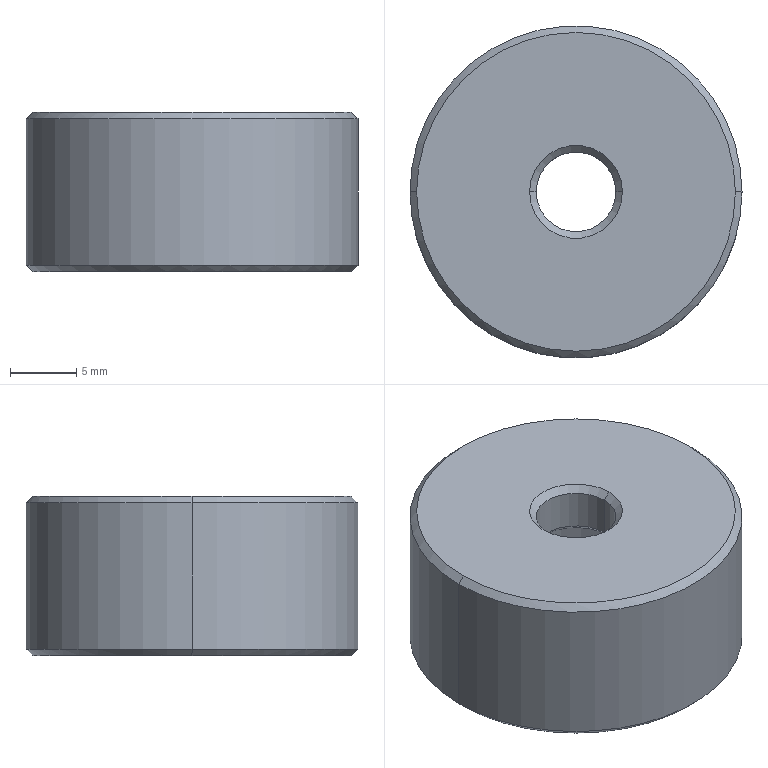Part | SolidWorks | features Chamfer 1, Cut 1, Extrusion 1 | 1 solid | 19 faces | box 25 x 25 x 12 mm | volume 4138 mm3 | cone 10 | cylinder 6 | plane 3 | commonest cylinder face diameters 6 x2 16 x2 25 x2
STEP:
#1=CARTESIAN_POINT('',(-12.,0.,-6.));
#2=VERTEX_POINT('',#1);
#3=CARTESIAN_POINT('',(12.,0.,-6.));
#4=VERTEX_POINT('',#3);
#5=CARTESIAN_POINT('',(0.,0.,-6.));
#6=DIRECTION('',(0.,0.,-1.));
#7=DIRECTION('',(1.,0.,0.));
#8=AXIS2_PLACEMENT_3D('',#5,#6,#7);
#9=CIRCLE('',#8,12.);
#10=EDGE_CURVE('',#2,#4,#9,.T.);
#11=ORIENTED_EDGE('',*,*,#10,.F.);
#12=CARTESIAN_POINT('',(-12.5,0.,-5.5));
#13=VERTEX_POINT('',#12);
#14=CARTESIAN_POINT('',(-12.5,0.,-5.5));
#15=DIRECTION('',(-0.7071,0.,0.7071));
#16=VECTOR('',#15,1000.);
#17=LINE('',#14,#16);
#18=EDGE_CURVE('',#2,#13,#17,.T.);
#19=ORIENTED_EDGE('',*,*,#18,.T.);
#20=CARTESIAN_POINT('',(12.5,0.,-5.5));
#21=VERTEX_POINT('',#20);
#22=CARTESIAN_POINT('',(0.,0.,-5.5));
#23=DIRECTION('',(0.,0.,1.));
#24=DIRECTION('',(1.,0.,0.));
#25=AXIS2_PLACEMENT_3D('',#22,#23,#24);
#26=CIRCLE('',#25,12.5);
#27=EDGE_CURVE('',#21,#13,#26,.T.);
#28=ORIENTED_EDGE('',*,*,#27,.F.);
#29=CARTESIAN_POINT('',(12.5,0.,-5.5));
#30=DIRECTION('',(0.7071,0.,0.7071));
#31=VECTOR('',#30,1000.);
#32=LINE('',#29,#31);
#33=EDGE_CURVE('',#4,#21,#32,.T.);
#34=ORIENTED_EDGE('',*,*,#33,.F.);
#35=EDGE_LOOP('',(#11,#19,#28,#34));
#36=FACE_OUTER_BOUND('',#35,.T.);
#37=CARTESIAN_POINT('',(0.,0.,-5.5));
#38=DIRECTION('',(0.,0.,1.));
#39=DIRECTION('',(1.,0.,0.));
#40=AXIS2_PLACEMENT_3D('',#37,#38,#39);
#41=CONICAL_SURFACE('',#40,12.5,0.7854);
#42=ADVANCED_FACE('',(#36),#41,.T.);
#43=CARTESIAN_POINT('',(12.,0.,6.));
#44=VERTEX_POINT('',#43);
#45=CARTESIAN_POINT('',(-12.,0.,6.));
#46=VERTEX_POINT('',#45);
#47=CARTESIAN_POINT('',(0.,0.,6.));
#48=DIRECTION('',(0.,0.,1.));
#49=DIRECTION('',(1.,0.,0.));
#50=AXIS2_PLACEMENT_3D('',#47,#48,#49);
#51=CIRCLE('',#50,12.);
#52=EDGE_CURVE('',#44,#46,#51,.T.);
#53=ORIENTED_EDGE('',*,*,#52,.F.);
#54=CARTESIAN_POINT('',(12.5,0.,5.5));
#55=VERTEX_POINT('',#54);
#56=CARTESIAN_POINT('',(12.,0.,6.));
#57=DIRECTION('',(0.7071,0.,-0.7071));
#58=VECTOR('',#57,1000.);
#59=LINE('',#56,#58);
#60=EDGE_CURVE('',#44,#55,#59,.T.);
#61=ORIENTED_EDGE('',*,*,#60,.T.);
#62=CARTESIAN_POINT('',(-12.5,0.,5.5));
#63=VERTEX_POINT('',#62);
#64=CARTESIAN_POINT('',(0.,0.,5.5));
#65=DIRECTION('',(0.,0.,-1.));
#66=DIRECTION('',(1.,0.,0.));
#67=AXIS2_PLACEMENT_3D('',#64,#65,#66);
#68=CIRCLE('',#67,12.5);
#69=EDGE_CURVE('',#63,#55,#68,.T.);
#70=ORIENTED_EDGE('',*,*,#69,.F.);
#71=CARTESIAN_POINT('',(-12.,0.,6.));
#72=DIRECTION('',(-0.7071,0.,-0.7071));
#73=VECTOR('',#72,1000.);
#74=LINE('',#71,#73);
#75=EDGE_CURVE('',#46,#63,#74,.T.);
#76=ORIENTED_EDGE('',*,*,#75,.F.);
#77=EDGE_LOOP('',(#53,#61,#70,#76));
#78=FACE_OUTER_BOUND('',#77,.T.);
#79=CARTESIAN_POINT('',(0.,0.,6.));
#80=DIRECTION('',(0.,0.,-1.));
#81=DIRECTION('',(-1.,0.,0.));
#82=AXIS2_PLACEMENT_3D('',#79,#80,#81);
#83=CONICAL_SURFACE('',#82,12.,0.7854);
#84=ADVANCED_FACE('',(#78),#83,.T.);
#85=CARTESIAN_POINT('',(8.,0.,-5.5));
#86=VERTEX_POINT('',#85);
#87=CARTESIAN_POINT('',(-8.,0.,-5.5));
#88=VERTEX_POINT('',#87);
#89=CARTESIAN_POINT('',(0.,0.,-5.5));
#90=DIRECTION('',(0.,0.,-1.));
#91=DIRECTION('',(1.,0.,0.));
#92=AXIS2_PLACEMENT_3D('',#89,#90,#91);
#93=CIRCLE('',#92,8.);
#94=EDGE_CURVE('',#86,#88,#93,.T.);
#95=ORIENTED_EDGE('',*,*,#94,.F.);
#96=CARTESIAN_POINT('',(8.5,0.,-6.));
#97=VERTEX_POINT('',#96);
#98=CARTESIAN_POINT('',(8.,0.,-5.5));
#99=DIRECTION('',(0.7071,0.,-0.7071));
#100=VECTOR('',#99,1000.);
#101=LINE('',#98,#100);
#102=EDGE_CURVE('',#86,#97,#101,.T.);
#103=ORIENTED_EDGE('',*,*,#102,.T.);
#104=CARTESIAN_POINT('',(-8.5,0.,-6.));
#105=VERTEX_POINT('',#104);
#106=CARTESIAN_POINT('',(0.,0.,-6.));
#107=DIRECTION('',(0.,0.,1.));
#108=DIRECTION('',(1.,0.,0.));
#109=AXIS2_PLACEMENT_3D('',#106,#107,#108);
#110=CIRCLE('',#109,8.5);
#111=EDGE_CURVE('',#105,#97,#110,.T.);
#112=ORIENTED_EDGE('',*,*,#111,.F.);
#113=CARTESIAN_POINT('',(-8.,0.,-5.5));
#114=DIRECTION('',(-0.7071,0.,-0.7071));
#115=VECTOR('',#114,1000.);
#116=LINE('',#113,#115);
#117=EDGE_CURVE('',#88,#105,#116,.T.);
#118=ORIENTED_EDGE('',*,*,#117,.F.);
#119=EDGE_LOOP('',(#95,#103,#112,#118));
#120=FACE_OUTER_BOUND('',#119,.T.);
#121=CARTESIAN_POINT('',(0.,0.,-5.5));
#122=DIRECTION('',(0.,0.,-1.));
#123=DIRECTION('',(-1.,0.,0.));
#124=AXIS2_PLACEMENT_3D('',#121,#122,#123);
#125=CONICAL_SURFACE('',#124,8.,0.7854);
#126=ADVANCED_FACE('',(#120),#125,.F.);
#127=CARTESIAN_POINT('',(3.,0.,2.5));
#128=VERTEX_POINT('',#127);
#129=CARTESIAN_POINT('',(-3.,0.,2.5));
#130=VERTEX_POINT('',#129);
#131=CARTESIAN_POINT('',(0.,0.,2.5));
#132=DIRECTION('',(0.,0.,-1.));
#133=DIRECTION('',(-1.,0.,0.));
#134=AXIS2_PLACEMENT_3D('',#131,#132,#133);
#135=CIRCLE('',#134,3.);
#136=EDGE_CURVE('',#128,#130,#135,.T.);
#137=ORIENTED_EDGE('',*,*,#136,.F.);
#138=CARTESIAN_POINT('',(3.5,0.,2.));
#139=VERTEX_POINT('',#138);
#140=CARTESIAN_POINT('',(3.,0.,2.5));
#141=DIRECTION('',(0.7071,0.,-0.7071));
#142=VECTOR('',#141,1000.);
#143=LINE('',#140,#142);
#144=EDGE_CURVE('',#128,#139,#143,.T.);
#145=ORIENTED_EDGE('',*,*,#144,.T.);
#146=CARTESIAN_POINT('',(-3.5,0.,2.));
#147=VERTEX_POINT('',#146);
#148=CARTESIAN_POINT('',(0.,0.,2.));
#149=DIRECTION('',(0.,0.,1.));
#150=DIRECTION('',(-1.,0.,0.));
#151=AXIS2_PLACEMENT_3D('',#148,#149,#150);
#152=CIRCLE('',#151,3.5);
#153=EDGE_CURVE('',#147,#139,#152,.T.);
#154=ORIENTED_EDGE('',*,*,#153,.F.);
#155=CARTESIAN_POINT('',(-3.,0.,2.5));
#156=DIRECTION('',(-0.7071,0.,-0.7071));
#157=VECTOR('',#156,1000.);
#158=LINE('',#155,#157);
#159=EDGE_CURVE('',#130,#147,#158,.T.);
#160=ORIENTED_EDGE('',*,*,#159,.F.);
#161=EDGE_LOOP('',(#137,#145,#154,#160));
#162=FACE_OUTER_BOUND('',#161,.T.);
#163=CARTESIAN_POINT('',(0.,0.,2.5));
#164=DIRECTION('',(0.,0.,-1.));
#165=DIRECTION('',(-1.,0.,0.));
#166=AXIS2_PLACEMENT_3D('',#163,#164,#165);
#167=CONICAL_SURFACE('',#166,3.,0.7854);
#168=ADVANCED_FACE('',(#162),#167,.F.);
#169=CARTESIAN_POINT('',(-3.,0.,5.5));
#170=VERTEX_POINT('',#169);
#171=CARTESIAN_POINT('',(3.,0.,5.5));
#172=VERTEX_POINT('',#171);
#173=CARTESIAN_POINT('',(0.,0.,5.5));
#174=DIRECTION('',(0.,0.,1.));
#175=DIRECTION('',(1.,0.,0.));
#176=AXIS2_PLACEMENT_3D('',#173,#174,#175);
#177=CIRCLE('',#176,3.);
#178=EDGE_CURVE('',#170,#172,#177,.T.);
#179=ORIENTED_EDGE('',*,*,#178,.F.);
#180=CARTESIAN_POINT('',(-3.5,0.,6.));
#181=VERTEX_POINT('',#180);
#182=CARTESIAN_POINT('',(-3.,0.,5.5));
#183=DIRECTION('',(-0.7071,0.,0.7071));
#184=VECTOR('',#183,1000.);
#185=LINE('',#182,#184);
#186=EDGE_CURVE('',#170,#181,#185,.T.);
#187=ORIENTED_EDGE('',*,*,#186,.T.);
#188=CARTESIAN_POINT('',(3.5,0.,6.));
#189=VERTEX_POINT('',#188);
#190=CARTESIAN_POINT('',(0.,0.,6.));
#191=DIRECTION('',(0.,0.,-1.));
#192=DIRECTION('',(1.,0.,0.));
#193=AXIS2_PLACEMENT_3D('',#190,#191,#192);
#194=CIRCLE('',#193,3.5);
#195=EDGE_CURVE('',#189,#181,#194,.T.);
#196=ORIENTED_EDGE('',*,*,#195,.F.);
#197=CARTESIAN_POINT('',(3.,0.,5.5));
#198=DIRECTION('',(0.7071,0.,0.7071));
#199=VECTOR('',#198,1000.);
#200=LINE('',#197,#199);
#201=EDGE_CURVE('',#172,#189,#200,.T.);
#202=ORIENTED_EDGE('',*,*,#201,.F.);
#203=EDGE_LOOP('',(#179,#187,#196,#202));
#204=FACE_OUTER_BOUND('',#203,.T.);
#205=CARTESIAN_POINT('',(0.,0.,5.5));
#206=DIRECTION('',(0.,0.,1.));
#207=DIRECTION('',(1.,0.,0.));
#208=AXIS2_PLACEMENT_3D('',#205,#206,#207);
#209=CONICAL_SURFACE('',#208,3.,0.7854);
#210=ADVANCED_FACE('',(#204),#209,.F.);
#211=CARTESIAN_POINT('',(8.,0.,2.));
#212=VERTEX_POINT('',#211);
#213=CARTESIAN_POINT('',(-8.,0.,2.));
#214=VERTEX_POINT('',#213);
#215=CARTESIAN_POINT('',(0.,0.,2.));
#216=DIRECTION('',(0.,0.,-1.));
#217=DIRECTION('',(-1.,0.,0.));
#218=AXIS2_PLACEMENT_3D('',#215,#216,#217);
#219=CIRCLE('',#218,8.);
#220=EDGE_CURVE('',#212,#214,#219,.T.);
#221=ORIENTED_EDGE('',*,*,#220,.F.);
#222=CARTESIAN_POINT('',(8.,0.,2.));
#223=DIRECTION('',(0.,0.,-1.));
#224=VECTOR('',#223,1000.);
#225=LINE('',#222,#224);
#226=EDGE_CURVE('',#212,#86,#225,.T.);
#227=ORIENTED_EDGE('',*,*,#226,.T.);
#228=ORIENTED_EDGE('',*,*,#94,.T.);
#229=CARTESIAN_POINT('',(-8.,0.,2.));
#230=DIRECTION('',(0.,0.,-1.));
#231=VECTOR('',#230,1000.);
#232=LINE('',#229,#231);
#233=EDGE_CURVE('',#214,#88,#232,.T.);
#234=ORIENTED_EDGE('',*,*,#233,.F.);
#235=EDGE_LOOP('',(#221,#227,#228,#234));
#236=FACE_OUTER_BOUND('',#235,.T.);
#237=CARTESIAN_POINT('',(0.,0.,2.));
#238=DIRECTION('',(0.,0.,-1.));
#239=DIRECTION('',(-1.,0.,0.));
#240=AXIS2_PLACEMENT_3D('',#237,#238,#239);
#241=CYLINDRICAL_SURFACE('',#240,8.);
#242=ADVANCED_FACE('',(#236),#241,.F.);
#243=ORIENTED_EDGE('',*,*,#69,.T.);
#244=CARTESIAN_POINT('',(12.5,0.,6.));
#245=DIRECTION('',(0.,0.,-1.));
#246=VECTOR('',#245,1000.);
#247=LINE('',#244,#246);
#248=EDGE_CURVE('',#55,#21,#247,.T.);
#249=ORIENTED_EDGE('',*,*,#248,.T.);
#250=ORIENTED_EDGE('',*,*,#27,.T.);
#251=CARTESIAN_POINT('',(-12.5,0.,6.));
#252=DIRECTION('',(0.,0.,-1.));
#253=VECTOR('',#252,1000.);
#254=LINE('',#251,#253);
#255=EDGE_CURVE('',#63,#13,#254,.T.);
#256=ORIENTED_EDGE('',*,*,#255,.F.);
#257=EDGE_LOOP('',(#243,#249,#250,#256));
#258=FACE_OUTER_BOUND('',#257,.T.);
#259=CARTESIAN_POINT('',(0.,0.,6.));
#260=DIRECTION('',(0.,0.,-1.));
#261=DIRECTION('',(-1.,0.,0.));
#262=AXIS2_PLACEMENT_3D('',#259,#260,#261);
#263=CYLINDRICAL_SURFACE('',#262,12.5);
#264=ADVANCED_FACE('',(#258),#263,.T.);
#265=ORIENTED_EDGE('',*,*,#178,.T.);
#266=CARTESIAN_POINT('',(3.,0.,6.));
#267=DIRECTION('',(0.,0.,-1.));
#268=VECTOR('',#267,1000.);
#269=LINE('',#266,#268);
#270=EDGE_CURVE('',#172,#128,#269,.T.);
#271=ORIENTED_EDGE('',*,*,#270,.T.);
#272=ORIENTED_EDGE('',*,*,#136,.T.);
#273=CARTESIAN_POINT('',(-3.,0.,6.));
#274=DIRECTION('',(0.,0.,-1.));
#275=VECTOR('',#274,1000.);
#276=LINE('',#273,#275);
#277=EDGE_CURVE('',#170,#130,#276,.T.);
#278=ORIENTED_EDGE('',*,*,#277,.F.);
#279=EDGE_LOOP('',(#265,#271,#272,#278));
#280=FACE_OUTER_BOUND('',#279,.T.);
#281=CARTESIAN_POINT('',(0.,0.,6.));
#282=DIRECTION('',(0.,0.,-1.));
#283=DIRECTION('',(-1.,0.,0.));
#284=AXIS2_PLACEMENT_3D('',#281,#282,#283);
#285=CYLINDRICAL_SURFACE('',#284,3.);
#286=ADVANCED_FACE('',(#280),#285,.F.);
#287=ORIENTED_EDGE('',*,*,#270,.F.);
#288=CARTESIAN_POINT('',(0.,0.,5.5));
#289=DIRECTION('',(0.,0.,1.));
#290=DIRECTION('',(1.,0.,0.));
#291=AXIS2_PLACEMENT_3D('',#288,#289,#290);
#292=CIRCLE('',#291,3.);
#293=EDGE_CURVE('',#172,#170,#292,.T.);
#294=ORIENTED_EDGE('',*,*,#293,.T.);
#295=ORIENTED_EDGE('',*,*,#277,.T.);
#296=CARTESIAN_POINT('',(0.,0.,2.5));
#297=DIRECTION('',(0.,0.,-1.));
#298=DIRECTION('',(-1.,0.,0.));
#299=AXIS2_PLACEMENT_3D('',#296,#297,#298);
#300=CIRCLE('',#299,3.);
#301=EDGE_CURVE('',#130,#128,#300,.T.);
#302=ORIENTED_EDGE('',*,*,#301,.T.);
#303=EDGE_LOOP('',(#287,#294,#295,#302));
#304=FACE_OUTER_BOUND('',#303,.T.);
#305=CARTESIAN_POINT('',(0.,0.,6.));
#306=DIRECTION('',(0.,0.,-1.));
#307=DIRECTION('',(-1.,0.,0.));
#308=AXIS2_PLACEMENT_3D('',#305,#306,#307);
#309=CYLINDRICAL_SURFACE('',#308,3.);
#310=ADVANCED_FACE('',(#304),#309,.F.);
#311=ORIENTED_EDGE('',*,*,#195,.T.);
#312=CARTESIAN_POINT('',(0.,0.,6.));
#313=DIRECTION('',(0.,0.,-1.));
#314=DIRECTION('',(1.,0.,0.));
#315=AXIS2_PLACEMENT_3D('',#312,#313,#314);
#316=CIRCLE('',#315,3.5);
#317=EDGE_CURVE('',#181,#189,#316,.T.);
#318=ORIENTED_EDGE('',*,*,#317,.T.);
#319=EDGE_LOOP('',(#311,#318));
#320=FACE_BOUND('',#319,.T.);
#321=CARTESIAN_POINT('',(0.,0.,6.));
#322=DIRECTION('',(0.,0.,1.));
#323=DIRECTION('',(1.,0.,0.));
#324=AXIS2_PLACEMENT_3D('',#321,#322,#323);
#325=CIRCLE('',#324,12.);
#326=EDGE_CURVE('',#46,#44,#325,.T.);
#327=ORIENTED_EDGE('',*,*,#326,.T.);
#328=ORIENTED_EDGE('',*,*,#52,.T.);
#329=EDGE_LOOP('',(#327,#328));
#330=FACE_OUTER_BOUND('',#329,.T.);
#331=CARTESIAN_POINT('',(0.,0.,6.));
#332=DIRECTION('',(0.,0.,1.));
#333=DIRECTION('',(1.,0.,0.));
#334=AXIS2_PLACEMENT_3D('',#331,#332,#333);
#335=PLANE('',#334);
#336=ADVANCED_FACE('',(#320,#330),#335,.T.);
#337=ORIENTED_EDGE('',*,*,#111,.T.);
#338=CARTESIAN_POINT('',(0.,0.,-6.));
#339=DIRECTION('',(0.,0.,1.));
#340=DIRECTION('',(1.,0.,0.));
#341=AXIS2_PLACEMENT_3D('',#338,#339,#340);
#342=CIRCLE('',#341,8.5);
#343=EDGE_CURVE('',#97,#105,#342,.T.);
#344=ORIENTED_EDGE('',*,*,#343,.T.);
#345=EDGE_LOOP('',(#337,#344));
#346=FACE_BOUND('',#345,.T.);
#347=CARTESIAN_POINT('',(0.,0.,-6.));
#348=DIRECTION('',(0.,0.,-1.));
#349=DIRECTION('',(1.,0.,0.));
#350=AXIS2_PLACEMENT_3D('',#347,#348,#349);
#351=CIRCLE('',#350,12.);
#352=EDGE_CURVE('',#4,#2,#351,.T.);
#353=ORIENTED_EDGE('',*,*,#352,.T.);
#354=ORIENTED_EDGE('',*,*,#10,.T.);
#355=EDGE_LOOP('',(#353,#354));
#356=FACE_OUTER_BOUND('',#355,.T.);
#357=CARTESIAN_POINT('',(0.,0.,-6.));
#358=DIRECTION('',(0.,0.,1.));
#359=DIRECTION('',(1.,0.,0.));
#360=AXIS2_PLACEMENT_3D('',#357,#358,#359);
#361=PLANE('',#360);
#362=ADVANCED_FACE('',(#346,#356),#361,.F.);
#363=ORIENTED_EDGE('',*,*,#248,.F.);
#364=CARTESIAN_POINT('',(0.,0.,5.5));
#365=DIRECTION('',(0.,0.,-1.));
#366=DIRECTION('',(1.,0.,0.));
#367=AXIS2_PLACEMENT_3D('',#364,#365,#366);
#368=CIRCLE('',#367,12.5);
#369=EDGE_CURVE('',#55,#63,#368,.T.);
#370=ORIENTED_EDGE('',*,*,#369,.T.);
#371=ORIENTED_EDGE('',*,*,#255,.T.);
#372=CARTESIAN_POINT('',(0.,0.,-5.5));
#373=DIRECTION('',(0.,0.,1.));
#374=DIRECTION('',(1.,0.,0.));
#375=AXIS2_PLACEMENT_3D('',#372,#373,#374);
#376=CIRCLE('',#375,12.5);
#377=EDGE_CURVE('',#13,#21,#376,.T.);
#378=ORIENTED_EDGE('',*,*,#377,.T.);
#379=EDGE_LOOP('',(#363,#370,#371,#378));
#380=FACE_OUTER_BOUND('',#379,.T.);
#381=CARTESIAN_POINT('',(0.,0.,6.));
#382=DIRECTION('',(0.,0.,-1.));
#383=DIRECTION('',(-1.,0.,0.));
#384=AXIS2_PLACEMENT_3D('',#381,#382,#383);
#385=CYLINDRICAL_SURFACE('',#384,12.5);
#386=ADVANCED_FACE('',(#380),#385,.T.);
#387=ORIENTED_EDGE('',*,*,#226,.F.);
#388=CARTESIAN_POINT('',(0.,0.,2.));
#389=DIRECTION('',(0.,0.,-1.));
#390=DIRECTION('',(-1.,0.,0.));
#391=AXIS2_PLACEMENT_3D('',#388,#389,#390);
#392=CIRCLE('',#391,8.);
#393=EDGE_CURVE('',#214,#212,#392,.T.);
#394=ORIENTED_EDGE('',*,*,#393,.F.);
#395=ORIENTED_EDGE('',*,*,#233,.T.);
#396=CARTESIAN_POINT('',(0.,0.,-5.5));
#397=DIRECTION('',(0.,0.,-1.));
#398=DIRECTION('',(1.,0.,0.));
#399=AXIS2_PLACEMENT_3D('',#396,#397,#398);
#400=CIRCLE('',#399,8.);
#401=EDGE_CURVE('',#88,#86,#400,.T.);
#402=ORIENTED_EDGE('',*,*,#401,.T.);
#403=EDGE_LOOP('',(#387,#394,#395,#402));
#404=FACE_OUTER_BOUND('',#403,.T.);
#405=CARTESIAN_POINT('',(0.,0.,2.));
#406=DIRECTION('',(0.,0.,-1.));
#407=DIRECTION('',(-1.,0.,0.));
#408=AXIS2_PLACEMENT_3D('',#405,#406,#407);
#409=CYLINDRICAL_SURFACE('',#408,8.);
#410=ADVANCED_FACE('',(#404),#409,.F.);
#411=ORIENTED_EDGE('',*,*,#153,.T.);
#412=CARTESIAN_POINT('',(0.,0.,2.));
#413=DIRECTION('',(0.,0.,1.));
#414=DIRECTION('',(-1.,0.,0.));
#415=AXIS2_PLACEMENT_3D('',#412,#413,#414);
#416=CIRCLE('',#415,3.5);
#417=EDGE_CURVE('',#139,#147,#416,.T.);
#418=ORIENTED_EDGE('',*,*,#417,.T.);
#419=EDGE_LOOP('',(#411,#418));
#420=FACE_BOUND('',#419,.T.);
#421=ORIENTED_EDGE('',*,*,#393,.T.);
#422=ORIENTED_EDGE('',*,*,#220,.T.);
#423=EDGE_LOOP('',(#421,#422));
#424=FACE_OUTER_BOUND('',#423,.T.);
#425=CARTESIAN_POINT('',(0.,0.,2.));
#426=DIRECTION('',(0.,0.,-1.));
#427=DIRECTION('',(-1.,0.,0.));
#428=AXIS2_PLACEMENT_3D('',#425,#426,#427);
#429=PLANE('',#428);
#430=ADVANCED_FACE('',(#420,#424),#429,.T.);
#431=ORIENTED_EDGE('',*,*,#186,.F.);
#432=ORIENTED_EDGE('',*,*,#293,.F.);
#433=ORIENTED_EDGE('',*,*,#201,.T.);
#434=ORIENTED_EDGE('',*,*,#317,.F.);
#435=EDGE_LOOP('',(#431,#432,#433,#434));
#436=FACE_OUTER_BOUND('',#435,.T.);
#437=CARTESIAN_POINT('',(0.,0.,5.5));
#438=DIRECTION('',(0.,0.,1.));
#439=DIRECTION('',(1.,0.,0.));
#440=AXIS2_PLACEMENT_3D('',#437,#438,#439);
#441=CONICAL_SURFACE('',#440,3.,0.7854);
#442=ADVANCED_FACE('',(#436),#441,.F.);
#443=ORIENTED_EDGE('',*,*,#144,.F.);
#444=ORIENTED_EDGE('',*,*,#301,.F.);
#445=ORIENTED_EDGE('',*,*,#159,.T.);
#446=ORIENTED_EDGE('',*,*,#417,.F.);
#447=EDGE_LOOP('',(#443,#444,#445,#446));
#448=FACE_OUTER_BOUND('',#447,.T.);
#449=CARTESIAN_POINT('',(0.,0.,2.5));
#450=DIRECTION('',(0.,0.,-1.));
#451=DIRECTION('',(-1.,0.,0.));
#452=AXIS2_PLACEMENT_3D('',#449,#450,#451);
#453=CONICAL_SURFACE('',#452,3.,0.7854);
#454=ADVANCED_FACE('',(#448),#453,.F.);
#455=ORIENTED_EDGE('',*,*,#102,.F.);
#456=ORIENTED_EDGE('',*,*,#401,.F.);
#457=ORIENTED_EDGE('',*,*,#117,.T.);
#458=ORIENTED_EDGE('',*,*,#343,.F.);
#459=EDGE_LOOP('',(#455,#456,#457,#458));
#460=FACE_OUTER_BOUND('',#459,.T.);
#461=CARTESIAN_POINT('',(0.,0.,-5.5));
#462=DIRECTION('',(0.,0.,-1.));
#463=DIRECTION('',(-1.,0.,0.));
#464=AXIS2_PLACEMENT_3D('',#461,#462,#463);
#465=CONICAL_SURFACE('',#464,8.,0.7854);
#466=ADVANCED_FACE('',(#460),#465,.F.);
#467=ORIENTED_EDGE('',*,*,#60,.F.);
#468=ORIENTED_EDGE('',*,*,#326,.F.);
#469=ORIENTED_EDGE('',*,*,#75,.T.);
#470=ORIENTED_EDGE('',*,*,#369,.F.);
#471=EDGE_LOOP('',(#467,#468,#469,#470));
#472=FACE_OUTER_BOUND('',#471,.T.);
#473=CARTESIAN_POINT('',(0.,0.,6.));
#474=DIRECTION('',(0.,0.,-1.));
#475=DIRECTION('',(-1.,0.,0.));
#476=AXIS2_PLACEMENT_3D('',#473,#474,#475);
#477=CONICAL_SURFACE('',#476,12.,0.7854);
#478=ADVANCED_FACE('',(#472),#477,.T.);
#479=ORIENTED_EDGE('',*,*,#18,.F.);
#480=ORIENTED_EDGE('',*,*,#352,.F.);
#481=ORIENTED_EDGE('',*,*,#33,.T.);
#482=ORIENTED_EDGE('',*,*,#377,.F.);
#483=EDGE_LOOP('',(#479,#480,#481,#482));
#484=FACE_OUTER_BOUND('',#483,.T.);
#485=CARTESIAN_POINT('',(0.,0.,-5.5));
#486=DIRECTION('',(0.,0.,1.));
#487=DIRECTION('',(1.,0.,0.));
#488=AXIS2_PLACEMENT_3D('',#485,#486,#487);
#489=CONICAL_SURFACE('',#488,12.5,0.7854);
#490=ADVANCED_FACE('',(#484),#489,.T.);
#491=CLOSED_SHELL('',(#42,#84,#126,#168,#210,#242,#264,#286,#310,#336,#362,#386,#410,#430,#442,#454,#466,#478,#490));
#492=MANIFOLD_SOLID_BREP('',#491);
#493=CARTESIAN_POINT('',(0.,0.,0.));
#494=DIRECTION('',(0.,0.,1.));
#495=DIRECTION('',(1.,0.,0.));
#496=AXIS2_PLACEMENT_3D('',#493,#494,#495);
#497=(LENGTH_UNIT()NAMED_UNIT(*)SI_UNIT(.MILLI.,.METRE.));
#498=UNCERTAINTY_MEASURE_WITH_UNIT(LENGTH_MEASURE(0.00001),#497,'','');
#499=(NAMED_UNIT(*)PLANE_ANGLE_UNIT()SI_UNIT($,.RADIAN.));
#500=(NAMED_UNIT(*)SI_UNIT($,.STERADIAN.)SOLID_ANGLE_UNIT());
#501=(GEOMETRIC_REPRESENTATION_CONTEXT(3)GLOBAL_UNCERTAINTY_ASSIGNED_CONTEXT((#498))GLOBAL_UNIT_ASSIGNED_CONTEXT((#497,#499,#500))REPRESENTATION_CONTEXT('',''));
#502=ADVANCED_BREP_SHAPE_REPRESENTATION('',(#492,#496),#501);